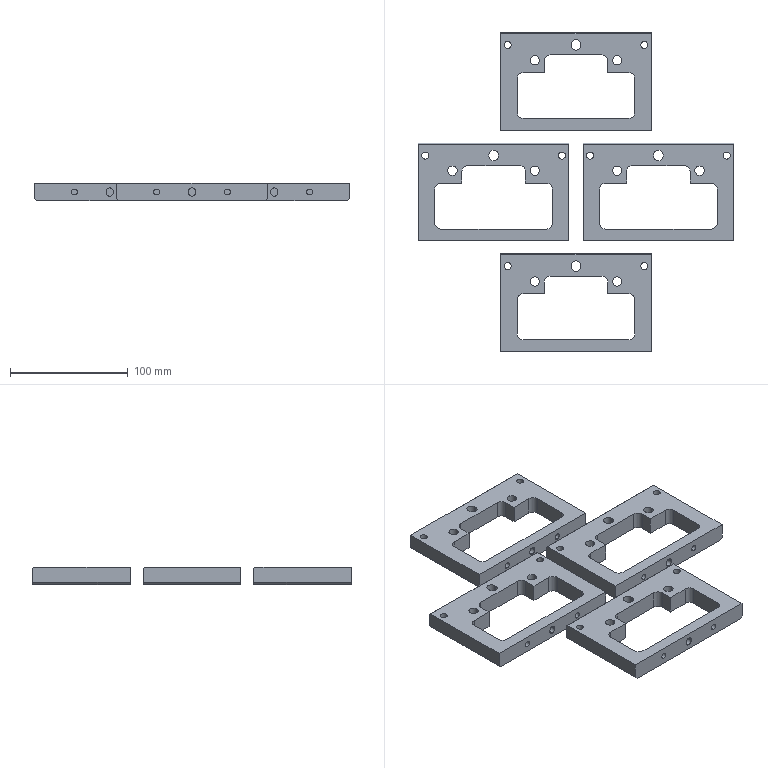NC program | NX | posted with a generic post | part box 268 x 271 x 15 mm
Lines 1 to 69 of 34527:
N10 G17 G21 G94 G90
(DRILLING , TOOL : D6A45)
N12 T07 M6
N14 G54
N16 G17 G0 G90 X58. Y-63. B0. C0. S5000 M3
N18 G43 Z30. H7
N20 G94 G81 G98 Z-1. F250. R3.
N22 X35. Y-76.
N24 X0. Y-62.5
N26 X-35. Y-76.
N28 X-58. Y-63.
N30 X-105. Y18.
N32 X-128. Y31.
N34 X-70. Y31.5
N36 X-35. Y18.
N38 X-12. Y31.
N40 X12.
N42 X35. Y18.
N44 X70. Y31.5
N46 X105. Y18.
N48 X128. Y31.
N50 X58. Y125.
N52 X35. Y112.
N54 X0. Y125.5
N56 X-35. Y112.
N58 X-58. Y125.
N60 G80
N62 G0 X-58. Y125. Z30.
N64 M5
(DRILLING_COPY , TOOL : 6.0ZT)
N66 T16 M6
N68 G54
N70 G17 G0 G90 X58. Y-63. B0. C0. S2000 M3
N72 G43 Z30. H16
N74 G94 G83 G98 Z-18.303 F200. Q2. R3.
N76 X12. Y31.
N78 X-12.
N80 X-58. Y-63.
N82 X-128. Y31.
N84 X-58. Y125.
N86 X58.
N88 X128. Y31.
N90 G80
N92 G0 X128. Y31. Z30.
(DRILLING_COPY_COPY , TOOL : 6.0ZT)
N94 X-105. Y18.
N96 G83 Z-18.303 F200. Q2. R3.
N98 X-70. Y31.5
N100 X-35. Y18.
N102 Y-76.
N104 X0. Y-62.5
N106 X35. Y-76.
N108 Y18.
N110 X70. Y31.5
N112 X105. Y18.
N114 X35. Y112.
N116 X0. Y125.5
N118 X-35. Y112.
N120 G80
N122 G0 X-35. Y112. Z30.
N124 M5